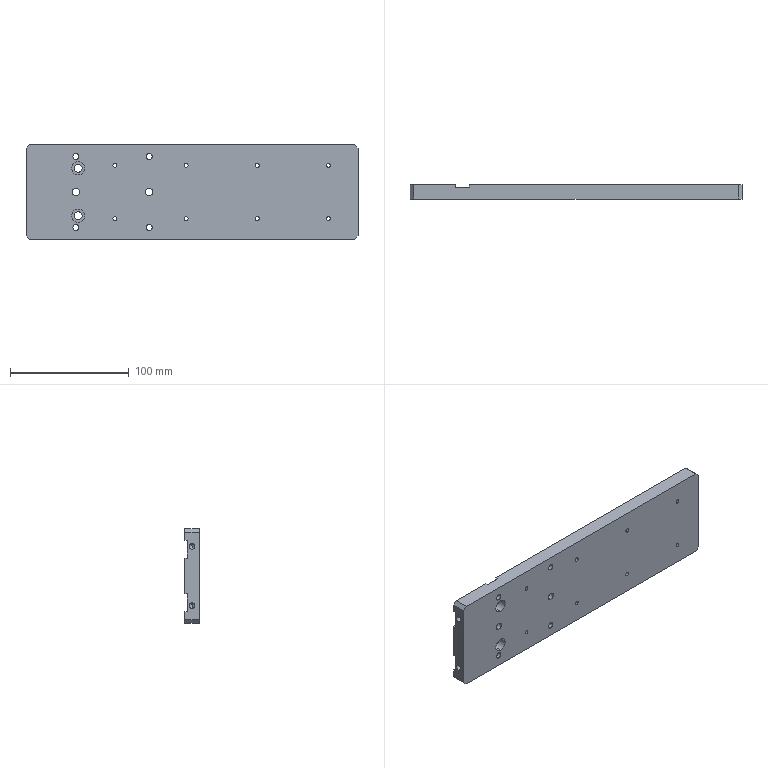Part | STEP file | PN_0040 | 1 solid | 86 faces | box 280 x 12 x 80 mm | volume 245567 mm3 | cylinder 44 | plane 34 | cone 8 | commonest cylinder face diameters 3.3 x16 5 x16 6 x4 6.6 x4 11 x4